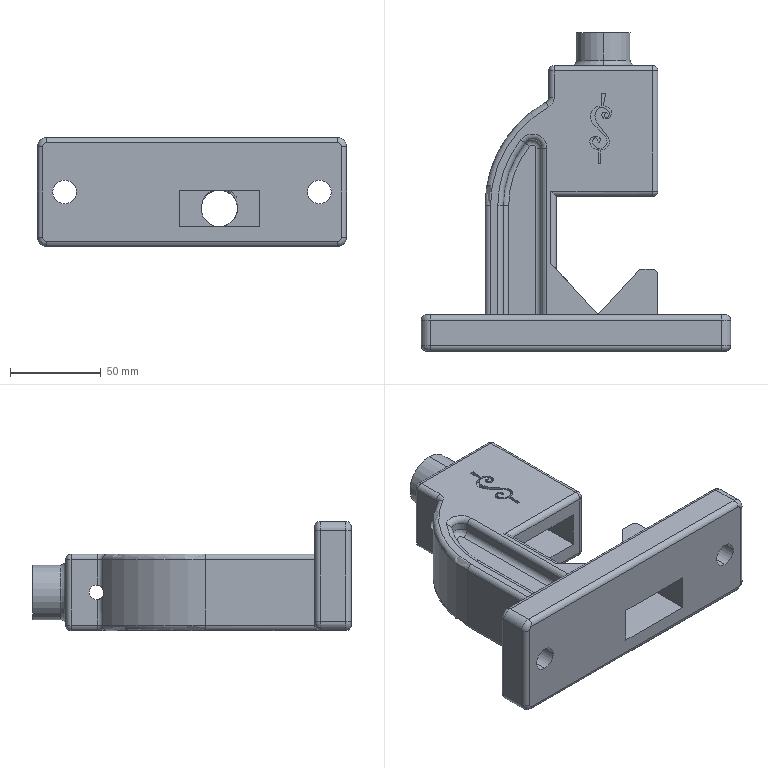Part | SolidWorks | features ICE 8, Fillet 2, Extrusion 1, Helix 1, MirrorPattern 1, SweepCut 1 | 1 solid | 169 faces | box 170 x 175 x 60 mm | volume 453597 mm3 | cylinder 70 | plane 42 | spline 29 | torus 22 | sphere 6 | commonest cylinder face diameters 6 x35 20 x16 10 x6 8 x4 13 x4 30 x2